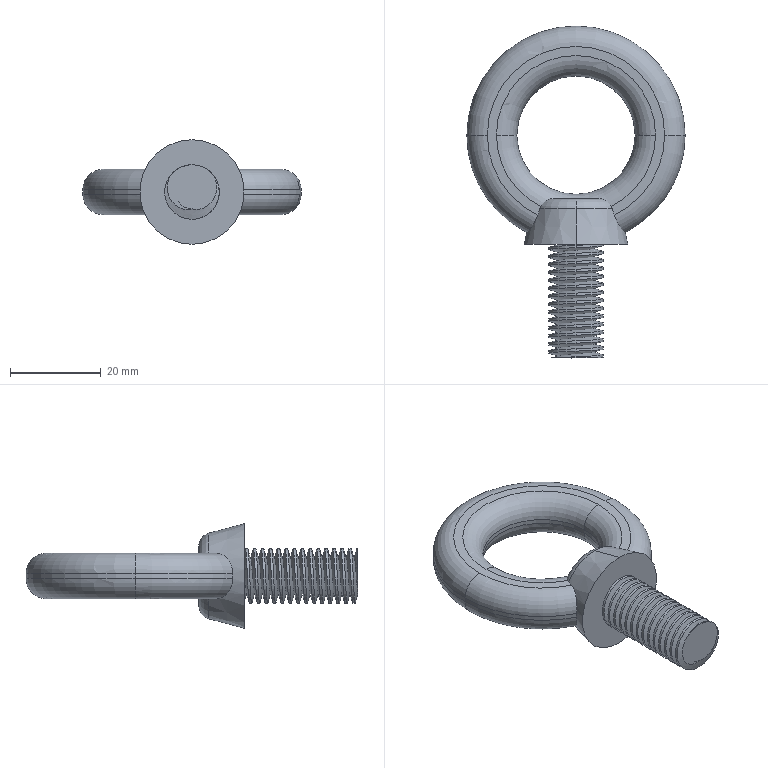Part | SolidWorks | features Boss 2, Fillet 2, Extrusion 1, Helix 1, SweepCut 1 | 1 solid | 58 faces | box 48 x 73 x 23 mm | volume 14602 mm3 | cylinder 35 | torus 13 | plane 6 | cone 2 | spline 2 | commonest cylinder face diameters 12 x30 48 x3 26 x2